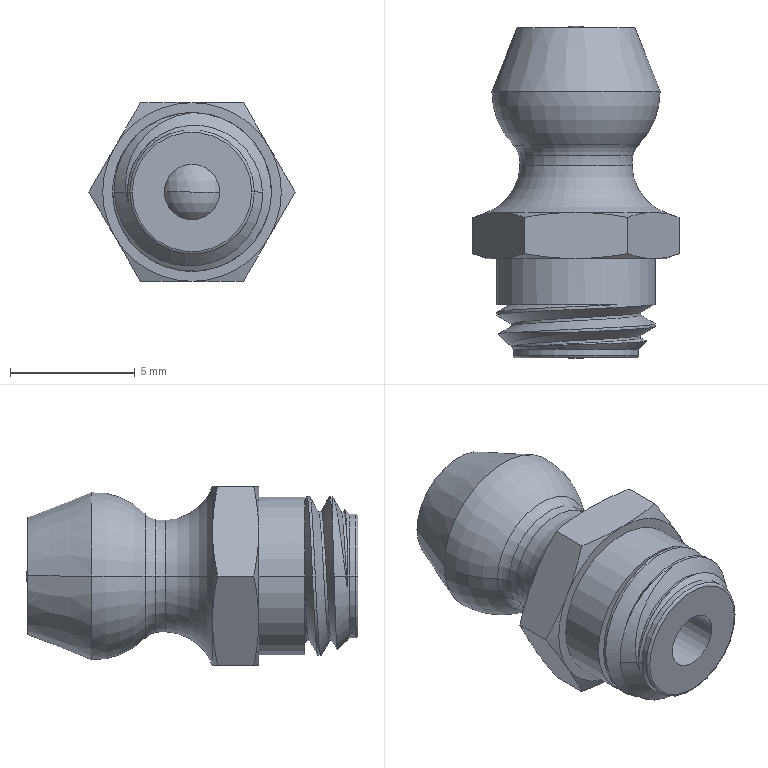Part | SolidWorks | features ICE 4, Revolution 3, Fillet 1, Helix 1, RevCut 1, Split 1, SweepCut 1 | 2 solids | 51 faces | box 8.249 x 13.277 x 7.144 mm | volume 337.025 mm3 | cone 18 | torus 10 | plane 10 | cylinder 8 | spline 3 | sphere 2 | commonest cylinder face diameters 6.35 x4 2.222 x2 4.989 x2